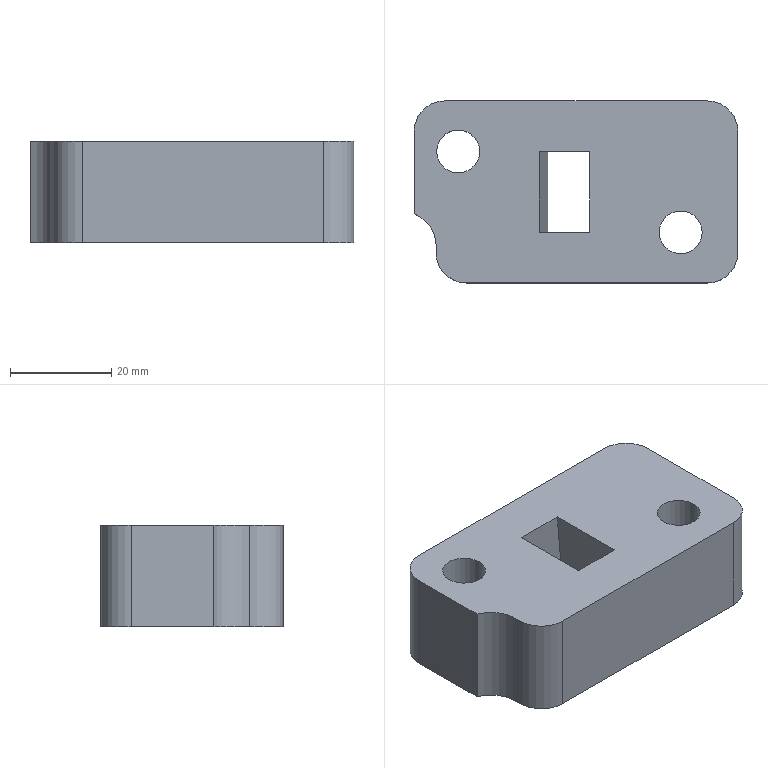Part | STEP file | solid 106 | 1 solid | 28 faces | box 64 x 36 x 20 mm | volume 37201 mm3 | plane 15 | cylinder 9 | other 4 | commonest cylinder face diameters 12 x4 14 x3 8.5 x2